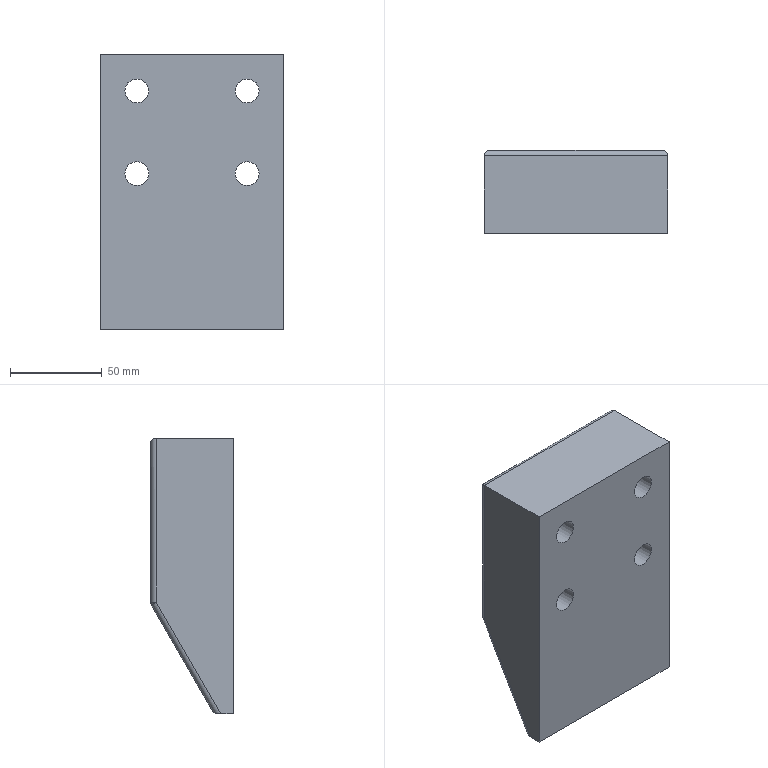Part | NX | features solid 2 | 1 solid | 47 faces | box 100 x 45 x 150 mm | volume 520948 mm3 | cylinder 19 | plane 11 | sphere 6 | torus 4 | spline 4 | cone 3 | commonest cylinder face diameters 6 x7 5 x4 13 x4 20 x4